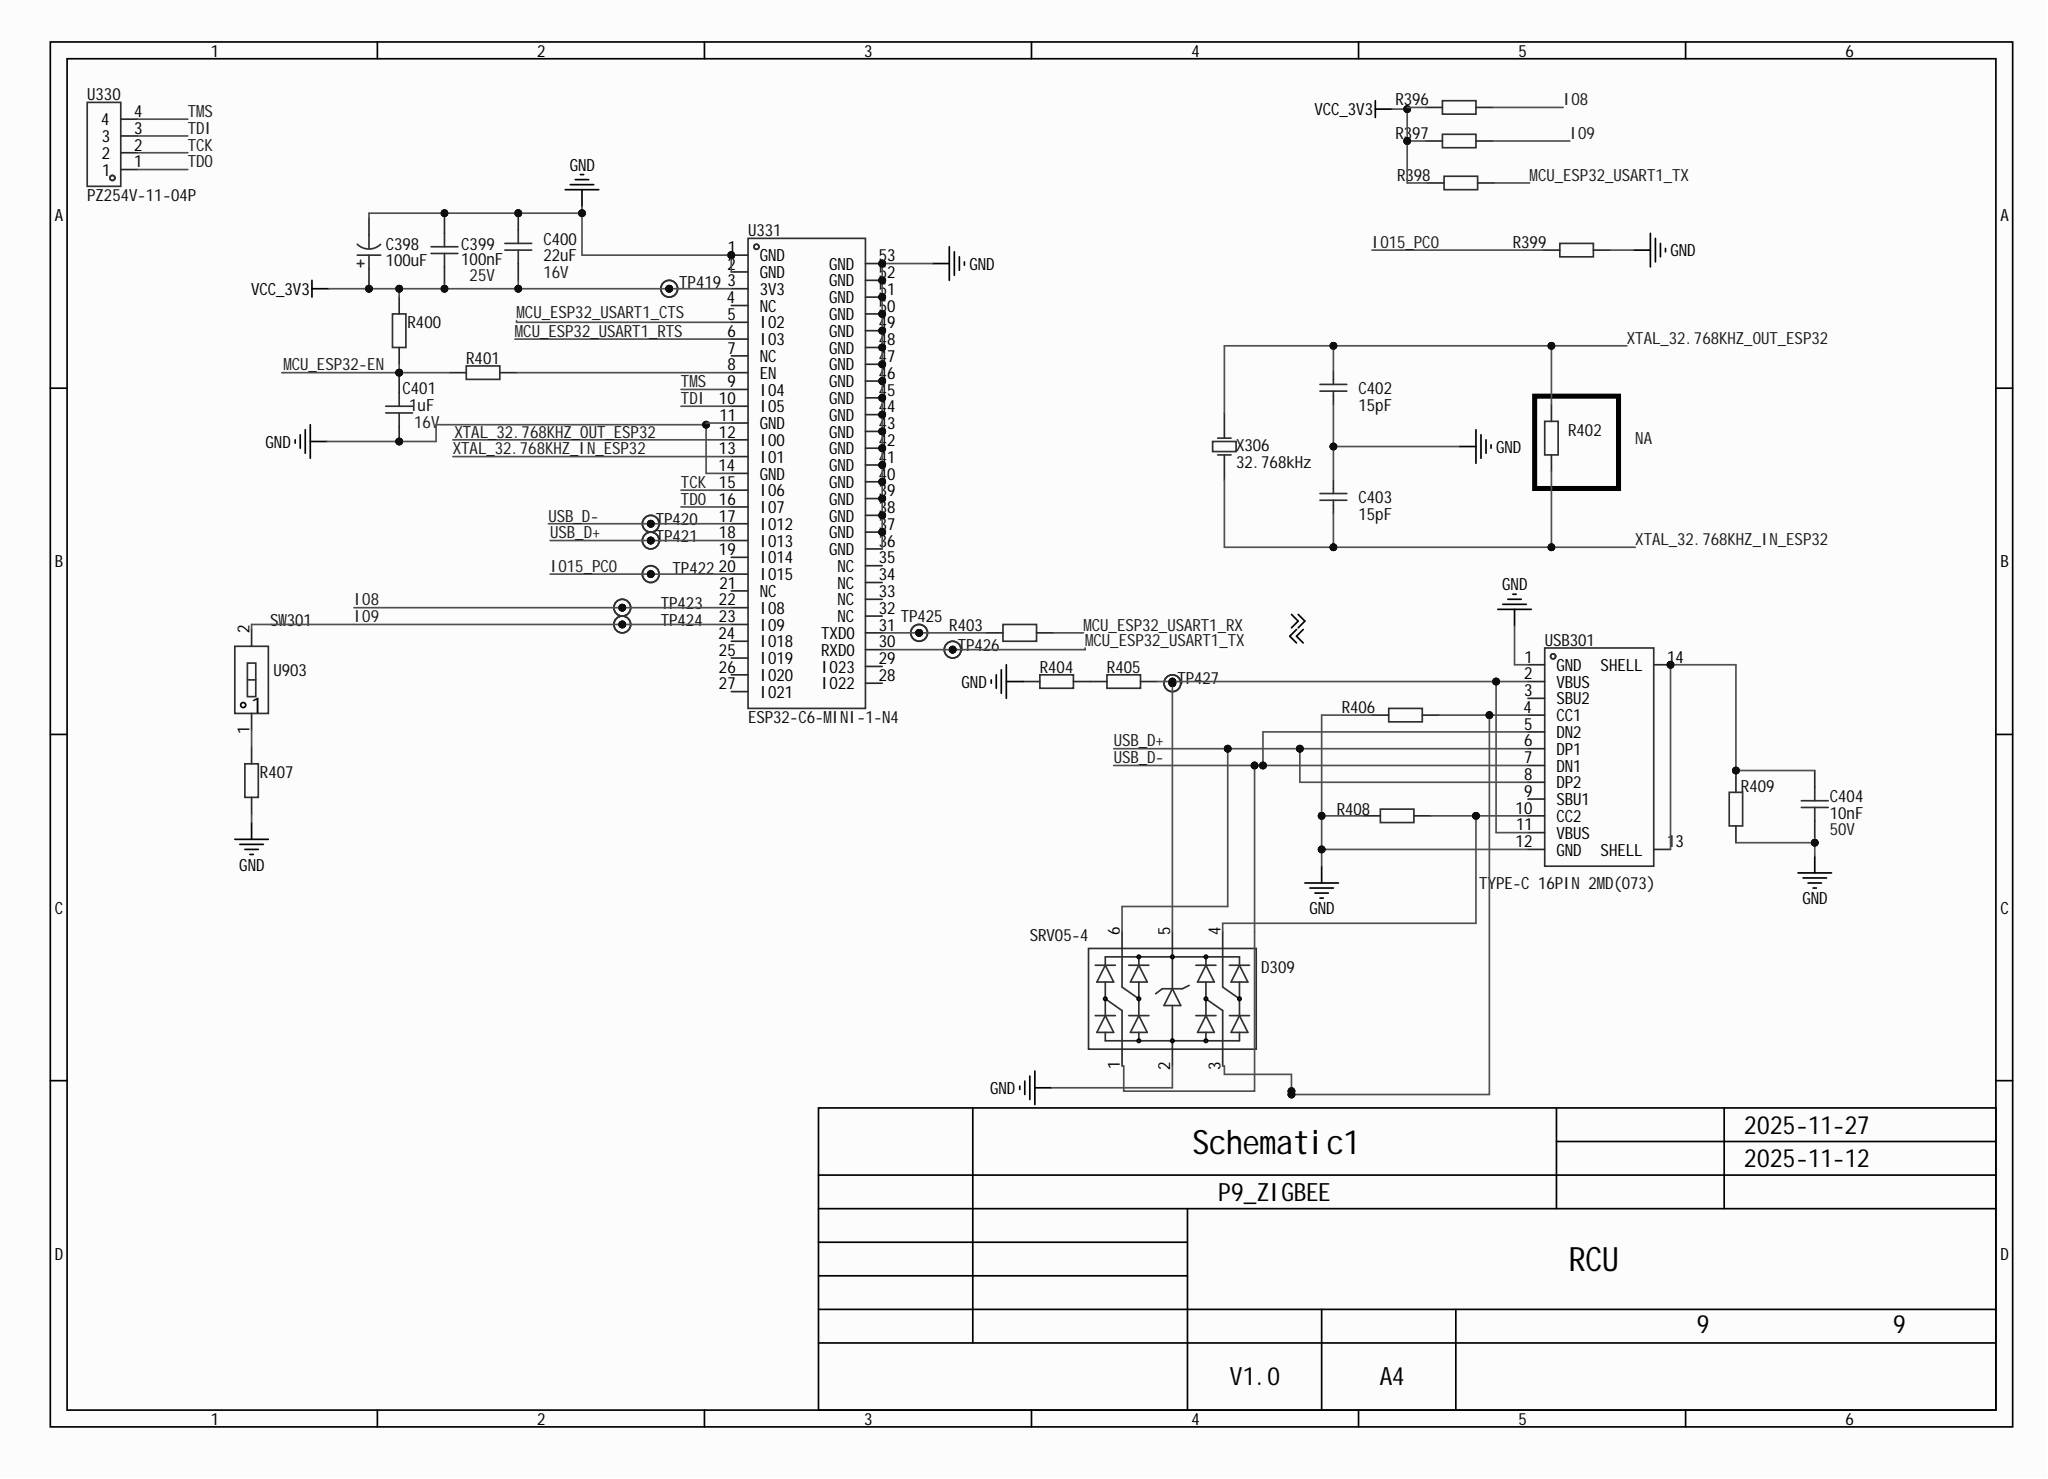Circuit board | Altium Designer | 424 parts | 202 nets | one sheet of the schematic
Parts on this sheet (reference | value | footprint):
C398 | 100uF | CAP-SMD_BD6.3-L6.6-W6.6-LS7.2-FD
C399 | 100nF | C0603
C400 | 22uF | C0603
C401 | 1uF | C0603
C402 | 15pF | C0402
C403 | 15pF | C0402
C404 | 10nF | C0603
D309 | SRV05-4 | SOT-23-6_L2.9-W1.6-P0.95-LS2.8-BL
R396 | R0603
R397 | R0603
R398 | R0603
R399 | R0603
R400 | R0603
R401 | R0603
R402 | R0402
R403 | R0603
R404 | R0603
R405 | R0603
R406 | R0603
R407 | R0603
R408 | R0603
R409 | R0402
SW301 | U903 | SW-SMD_2P-L3.5-W6.1-P2.54-LS9.8
TP419 | Test-Point-0.5mm
TP420 | Test-Point-0.5mm
TP421 | Test-Point-0.5mm
TP422 | Test-Point-0.5mm
TP423 | Test-Point-0.5mm
TP424 | Test-Point-0.5mm
TP425 | Test-Point-0.5mm
TP426 | Test-Point-0.5mm
TP427 | Test-Point-0.5mm
U330 | PZ254V-11-04P | HDR-TH_4P-P2.54-V-M
U331 | ESP32-C6-MINI-1-N4 | WIFIM-SMD_61P-L16.6-W13.2-P0.80-ESP32-C6-MINI-1-N4
USB301 | TYPE-C 16PIN 2MD(073) | USB-C-SMD_TYPE-C-6PIN-2MD-073
X306 | 32.768kHz | OSC-TH_BD3.1-P0.8-D0.3
Nets of these parts (net: part-pin ...):
XTAL_32.768KHZ_OUT_ESP32: C402-2 R402-2 X306-1 U331-12
XTAL_32.768KHZ_IN_ESP32: C403-1 R402-1 X306-2 U331-13
VCC_3V3: C398-1 C399-2 C400-1 R396-2 R397-2 R398-2 R400-2 TP419-1 U331-3
USB_D-: D309-1 TP420-1 USB301-5 USB301-7 U331-17
USB_D+: D309-6 TP421-1 USB301-6 USB301-8 U331-18
TMS: U330-4 U331-9
TDO: U330-1 U331-16
TDI: U330-3 U331-10
TCK: U330-2 U331-15
NetR407_2: R407-2 SW301-1
NetR404_1: R404-1 R405-1
NetR403_2: R403-2 TP425-1 U331-31
NetR401_2: R401-2 U331-8
NetD309_5: D309-5 R405-2 TP427-1 USB301-2 USB301-11
NetD309_4: D309-4 R408-2 USB301-10
NetD309_3: D309-3 R406-2 USB301-4
NetC404_2: C404-2 R409-2 USB301-13 USB301-14
MCU_ESP32_USART1_TX: R398-1 TP426-1 U331-30
MCU_ESP32_USART1_RX: R403-1
MCU_ESP32_USART1_RTS: U331-6
MCU_ESP32_USART1_CTS: U331-5
MCU_ESP32-EN: C401-2 R400-1 R401-1
IO15_PC0: R399-2 TP422-1 U331-20
IO9: R397-1 SW301-2 TP424-1 U331-23
IO8: R396-1 TP423-1 U331-22
GND: C398-2 C399-1 C400-2 C401-1 C402-1 C403-2 C404-1 D309-2 R399-1 R404-2 R406-1 R407-1 R408-1 R409-1 USB301-1 USB301-12 U331-1 U331-2 U331-11 U331-14 U331-36 U331-37 U331-38 U331-39 U331-40 U331-41 U331-42 U331-43 U331-44 U331-45 U331-46 U331-47 U331-48 U331-49 U331-50 U331-51 U331-52 U331-53